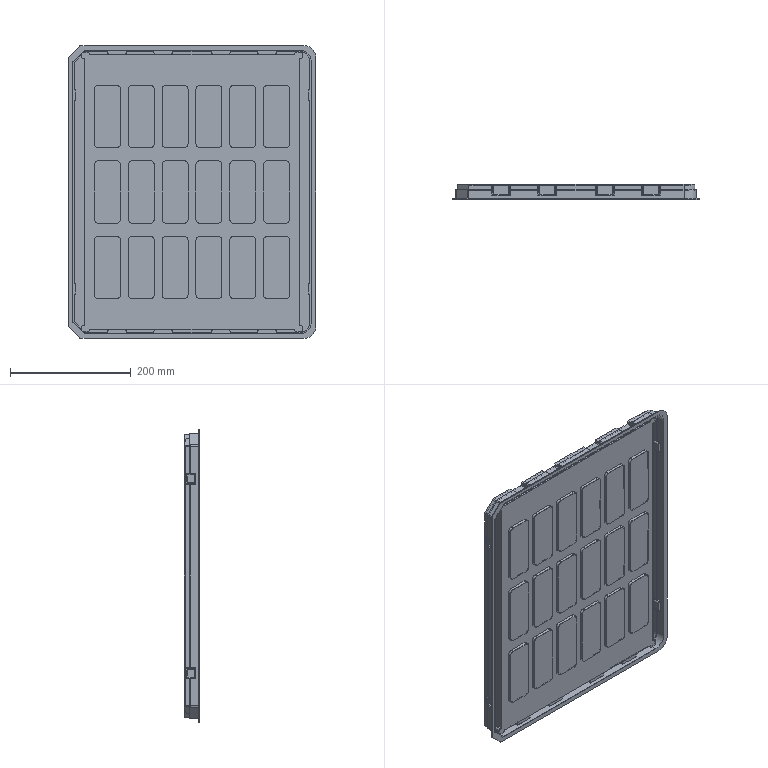Part | NX | 1 solid | 935 faces | box 410 x 25 x 485 mm | volume 443401 mm3 | plane 487 | cylinder 322 | spline 122 | cone 4 | commonest cylinder face diameters 10 x72 13 x72 3 x64 6 x32 2 x24 4 x20